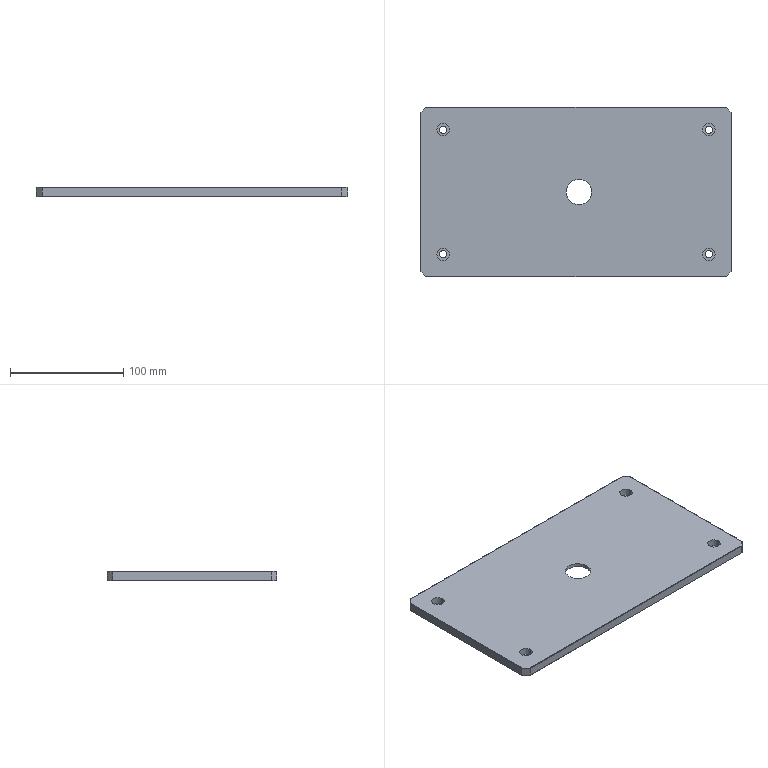Part | NX | 1 solid | 43 faces | box 275 x 150 x 8 mm | volume 300538 mm3 | plane 23 | cylinder 20 | commonest cylinder face diameters 6.4 x8 11 x8 22.5 x2 80 x2
STEP:
#1=CARTESIAN_POINT('',(0.3,4.7,0.));
#2=VERTEX_POINT('',#1);
#3=CARTESIAN_POINT('',(0.3,145.3,0.));
#4=VERTEX_POINT('',#3);
#5=CARTESIAN_POINT('',(0.3,75.,0.));
#6=DIRECTION('',(0.,1.,0.));
#7=VECTOR('',#6,1000.);
#8=LINE('',#5,#7);
#9=EDGE_CURVE('',#2,#4,#8,.T.);
#10=ORIENTED_EDGE('',*,*,#9,.T.);
#11=CARTESIAN_POINT('',(4.7,149.7,0.));
#12=VERTEX_POINT('',#11);
#13=CARTESIAN_POINT('',(5.,150.,0.));
#14=DIRECTION('',(-0.7071,-0.7071,0.));
#15=VECTOR('',#14,1000.);
#16=LINE('',#13,#15);
#17=EDGE_CURVE('',#12,#4,#16,.T.);
#18=ORIENTED_EDGE('',*,*,#17,.F.);
#19=CARTESIAN_POINT('',(270.3,149.7,0.));
#20=VERTEX_POINT('',#19);
#21=CARTESIAN_POINT('',(137.5,149.7,0.));
#22=DIRECTION('',(1.,0.,0.));
#23=VECTOR('',#22,1000.);
#24=LINE('',#21,#23);
#25=EDGE_CURVE('',#12,#20,#24,.T.);
#26=ORIENTED_EDGE('',*,*,#25,.T.);
#27=CARTESIAN_POINT('',(274.7,145.3,0.));
#28=VERTEX_POINT('',#27);
#29=CARTESIAN_POINT('',(275.,145.,0.));
#30=DIRECTION('',(-0.7071,0.7071,0.));
#31=VECTOR('',#30,1000.);
#32=LINE('',#29,#31);
#33=EDGE_CURVE('',#28,#20,#32,.T.);
#34=ORIENTED_EDGE('',*,*,#33,.F.);
#35=CARTESIAN_POINT('',(274.7,4.7,0.));
#36=VERTEX_POINT('',#35);
#37=CARTESIAN_POINT('',(274.7,75.,0.));
#38=DIRECTION('',(0.,-1.,0.));
#39=VECTOR('',#38,1000.);
#40=LINE('',#37,#39);
#41=EDGE_CURVE('',#28,#36,#40,.T.);
#42=ORIENTED_EDGE('',*,*,#41,.T.);
#43=CARTESIAN_POINT('',(270.3,0.3,0.));
#44=VERTEX_POINT('',#43);
#45=CARTESIAN_POINT('',(270.,0.,0.));
#46=DIRECTION('',(0.7071,0.7071,0.));
#47=VECTOR('',#46,1000.);
#48=LINE('',#45,#47);
#49=EDGE_CURVE('',#44,#36,#48,.T.);
#50=ORIENTED_EDGE('',*,*,#49,.F.);
#51=CARTESIAN_POINT('',(4.7,0.3,0.));
#52=VERTEX_POINT('',#51);
#53=CARTESIAN_POINT('',(137.5,0.3,0.));
#54=DIRECTION('',(-1.,0.,0.));
#55=VECTOR('',#54,1000.);
#56=LINE('',#53,#55);
#57=EDGE_CURVE('',#44,#52,#56,.T.);
#58=ORIENTED_EDGE('',*,*,#57,.T.);
#59=CARTESIAN_POINT('',(0.,5.,0.));
#60=DIRECTION('',(0.7071,-0.7071,0.));
#61=VECTOR('',#60,1000.);
#62=LINE('',#59,#61);
#63=EDGE_CURVE('',#2,#52,#62,.T.);
#64=ORIENTED_EDGE('',*,*,#63,.F.);
#65=EDGE_LOOP('',(#10,#18,#26,#34,#42,#50,#58,#64));
#66=FACE_BOUND('',#65,.T.);
#67=CARTESIAN_POINT('',(16.8,20.,0.));
#68=VERTEX_POINT('',#67);
#69=CARTESIAN_POINT('',(23.2,20.,0.));
#70=VERTEX_POINT('',#69);
#71=CARTESIAN_POINT('',(20.,20.,0.));
#72=DIRECTION('',(0.,0.,-1.));
#73=DIRECTION('',(-1.,0.,0.));
#74=AXIS2_PLACEMENT_3D('',#71,#72,#73);
#75=CIRCLE('',#74,3.2);
#76=EDGE_CURVE('',#68,#70,#75,.T.);
#77=ORIENTED_EDGE('',*,*,#76,.F.);
#78=CARTESIAN_POINT('',(20.,20.,0.));
#79=DIRECTION('',(0.,0.,-1.));
#80=DIRECTION('',(-1.,0.,0.));
#81=AXIS2_PLACEMENT_3D('',#78,#79,#80);
#82=CIRCLE('',#81,3.2);
#83=EDGE_CURVE('',#70,#68,#82,.T.);
#84=ORIENTED_EDGE('',*,*,#83,.F.);
#85=EDGE_LOOP('',(#77,#84));
#86=FACE_BOUND('',#85,.T.);
#87=CARTESIAN_POINT('',(258.2,130.,0.));
#88=VERTEX_POINT('',#87);
#89=CARTESIAN_POINT('',(251.8,130.,0.));
#90=VERTEX_POINT('',#89);
#91=CARTESIAN_POINT('',(255.,130.,0.));
#92=DIRECTION('',(0.,0.,-1.));
#93=DIRECTION('',(-1.,0.,0.));
#94=AXIS2_PLACEMENT_3D('',#91,#92,#93);
#95=CIRCLE('',#94,3.2);
#96=EDGE_CURVE('',#88,#90,#95,.T.);
#97=ORIENTED_EDGE('',*,*,#96,.F.);
#98=CARTESIAN_POINT('',(255.,130.,0.));
#99=DIRECTION('',(0.,0.,-1.));
#100=DIRECTION('',(-1.,0.,0.));
#101=AXIS2_PLACEMENT_3D('',#98,#99,#100);
#102=CIRCLE('',#101,3.2);
#103=EDGE_CURVE('',#90,#88,#102,.T.);
#104=ORIENTED_EDGE('',*,*,#103,.F.);
#105=EDGE_LOOP('',(#97,#104));
#106=FACE_BOUND('',#105,.T.);
#107=CARTESIAN_POINT('',(251.8,20.,0.));
#108=VERTEX_POINT('',#107);
#109=CARTESIAN_POINT('',(258.2,20.,0.));
#110=VERTEX_POINT('',#109);
#111=CARTESIAN_POINT('',(255.,20.,0.));
#112=DIRECTION('',(0.,0.,-1.));
#113=DIRECTION('',(-1.,0.,0.));
#114=AXIS2_PLACEMENT_3D('',#111,#112,#113);
#115=CIRCLE('',#114,3.2);
#116=EDGE_CURVE('',#108,#110,#115,.T.);
#117=ORIENTED_EDGE('',*,*,#116,.F.);
#118=CARTESIAN_POINT('',(255.,20.,0.));
#119=DIRECTION('',(0.,0.,-1.));
#120=DIRECTION('',(-1.,0.,0.));
#121=AXIS2_PLACEMENT_3D('',#118,#119,#120);
#122=CIRCLE('',#121,3.2);
#123=EDGE_CURVE('',#110,#108,#122,.T.);
#124=ORIENTED_EDGE('',*,*,#123,.F.);
#125=EDGE_LOOP('',(#117,#124));
#126=FACE_BOUND('',#125,.T.);
#127=CARTESIAN_POINT('',(180.,75.,0.));
#128=VERTEX_POINT('',#127);
#129=CARTESIAN_POINT('',(100.,75.,0.));
#130=VERTEX_POINT('',#129);
#131=CARTESIAN_POINT('',(140.,75.,0.));
#132=DIRECTION('',(0.,0.,-1.));
#133=DIRECTION('',(1.,0.,0.));
#134=AXIS2_PLACEMENT_3D('',#131,#132,#133);
#135=CIRCLE('',#134,40.);
#136=EDGE_CURVE('',#128,#130,#135,.T.);
#137=ORIENTED_EDGE('',*,*,#136,.F.);
#138=CARTESIAN_POINT('',(140.,75.,0.));
#139=DIRECTION('',(0.,0.,-1.));
#140=DIRECTION('',(1.,0.,0.));
#141=AXIS2_PLACEMENT_3D('',#138,#139,#140);
#142=CIRCLE('',#141,40.);
#143=EDGE_CURVE('',#130,#128,#142,.T.);
#144=ORIENTED_EDGE('',*,*,#143,.F.);
#145=EDGE_LOOP('',(#137,#144));
#146=FACE_BOUND('',#145,.T.);
#147=CARTESIAN_POINT('',(16.8,130.,0.));
#148=VERTEX_POINT('',#147);
#149=CARTESIAN_POINT('',(23.2,130.,0.));
#150=VERTEX_POINT('',#149);
#151=CARTESIAN_POINT('',(20.,130.,0.));
#152=DIRECTION('',(0.,0.,-1.));
#153=DIRECTION('',(-1.,0.,0.));
#154=AXIS2_PLACEMENT_3D('',#151,#152,#153);
#155=CIRCLE('',#154,3.2);
#156=EDGE_CURVE('',#148,#150,#155,.T.);
#157=ORIENTED_EDGE('',*,*,#156,.F.);
#158=CARTESIAN_POINT('',(20.,130.,0.));
#159=DIRECTION('',(0.,0.,-1.));
#160=DIRECTION('',(-1.,0.,0.));
#161=AXIS2_PLACEMENT_3D('',#158,#159,#160);
#162=CIRCLE('',#161,3.2);
#163=EDGE_CURVE('',#150,#148,#162,.T.);
#164=ORIENTED_EDGE('',*,*,#163,.F.);
#165=EDGE_LOOP('',(#157,#164));
#166=FACE_BOUND('',#165,.T.);
#167=CARTESIAN_POINT('',(0.,0.,0.));
#168=DIRECTION('',(0.,0.,1.));
#169=DIRECTION('',(1.,0.,0.));
#170=AXIS2_PLACEMENT_3D('',#167,#168,#169);
#171=PLANE('',#170);
#172=ADVANCED_FACE('',(#66,#86,#106,#126,#146,#166),#171,.F.);
#173=CARTESIAN_POINT('',(0.,5.,7.7));
#174=VERTEX_POINT('',#173);
#175=CARTESIAN_POINT('',(0.,145.,7.7));
#176=VERTEX_POINT('',#175);
#177=CARTESIAN_POINT('',(0.,75.,7.7));
#178=DIRECTION('',(0.,1.,0.));
#179=VECTOR('',#178,1000.);
#180=LINE('',#177,#179);
#181=EDGE_CURVE('',#174,#176,#180,.T.);
#182=ORIENTED_EDGE('',*,*,#181,.T.);
#183=CARTESIAN_POINT('',(0.,145.,0.3));
#184=VERTEX_POINT('',#183);
#185=CARTESIAN_POINT('',(0.,145.,8.));
#186=DIRECTION('',(0.,0.,-1.));
#187=VECTOR('',#186,1000.);
#188=LINE('',#185,#187);
#189=EDGE_CURVE('',#176,#184,#188,.T.);
#190=ORIENTED_EDGE('',*,*,#189,.T.);
#191=CARTESIAN_POINT('',(0.,5.,0.3));
#192=VERTEX_POINT('',#191);
#193=CARTESIAN_POINT('',(0.,75.,0.3));
#194=DIRECTION('',(0.,1.,0.));
#195=VECTOR('',#194,1000.);
#196=LINE('',#193,#195);
#197=EDGE_CURVE('',#192,#184,#196,.T.);
#198=ORIENTED_EDGE('',*,*,#197,.F.);
#199=CARTESIAN_POINT('',(0.,5.,8.));
#200=DIRECTION('',(0.,0.,-1.));
#201=VECTOR('',#200,1000.);
#202=LINE('',#199,#201);
#203=EDGE_CURVE('',#174,#192,#202,.T.);
#204=ORIENTED_EDGE('',*,*,#203,.F.);
#205=EDGE_LOOP('',(#182,#190,#198,#204));
#206=FACE_BOUND('',#205,.T.);
#207=CARTESIAN_POINT('',(0.,150.,0.));
#208=DIRECTION('',(-1.,0.,0.));
#209=DIRECTION('',(0.,0.,1.));
#210=AXIS2_PLACEMENT_3D('',#207,#208,#209);
#211=PLANE('',#210);
#212=ADVANCED_FACE('',(#206),#211,.T.);
#213=ORIENTED_EDGE('',*,*,#189,.F.);
#214=CARTESIAN_POINT('',(0.3,145.3,8.));
#215=VERTEX_POINT('',#214);
#216=CARTESIAN_POINT('',(-145.,0.,-137.3));
#217=DIRECTION('',(-0.5774,-0.5774,-0.5774));
#218=VECTOR('',#217,1000.);
#219=LINE('',#216,#218);
#220=EDGE_CURVE('',#215,#176,#219,.T.);
#221=ORIENTED_EDGE('',*,*,#220,.F.);
#222=CARTESIAN_POINT('',(4.7,149.7,8.));
#223=VERTEX_POINT('',#222);
#224=CARTESIAN_POINT('',(0.,145.,8.));
#225=DIRECTION('',(0.7071,0.7071,0.));
#226=VECTOR('',#225,1000.);
#227=LINE('',#224,#226);
#228=EDGE_CURVE('',#215,#223,#227,.T.);
#229=ORIENTED_EDGE('',*,*,#228,.T.);
#230=CARTESIAN_POINT('',(5.,150.,7.7));
#231=VERTEX_POINT('',#230);
#232=CARTESIAN_POINT('',(-145.,0.,157.7));
#233=DIRECTION('',(-0.5774,-0.5774,0.5774));
#234=VECTOR('',#233,1000.);
#235=LINE('',#232,#234);
#236=EDGE_CURVE('',#231,#223,#235,.T.);
#237=ORIENTED_EDGE('',*,*,#236,.F.);
#238=CARTESIAN_POINT('',(5.,150.,0.3));
#239=VERTEX_POINT('',#238);
#240=CARTESIAN_POINT('',(5.,150.,8.));
#241=DIRECTION('',(0.,0.,-1.));
#242=VECTOR('',#241,1000.);
#243=LINE('',#240,#242);
#244=EDGE_CURVE('',#231,#239,#243,.T.);
#245=ORIENTED_EDGE('',*,*,#244,.T.);
#246=CARTESIAN_POINT('',(-145.,0.,-149.7));
#247=DIRECTION('',(0.5774,0.5774,0.5774));
#248=VECTOR('',#247,1000.);
#249=LINE('',#246,#248);
#250=EDGE_CURVE('',#12,#239,#249,.T.);
#251=ORIENTED_EDGE('',*,*,#250,.F.);
#252=ORIENTED_EDGE('',*,*,#17,.T.);
#253=CARTESIAN_POINT('',(0.3,145.3,0.));
#254=DIRECTION('',(0.5774,0.5774,-0.5774));
#255=VECTOR('',#254,1000.);
#256=LINE('',#253,#255);
#257=EDGE_CURVE('',#184,#4,#256,.T.);
#258=ORIENTED_EDGE('',*,*,#257,.F.);
#259=EDGE_LOOP('',(#213,#221,#229,#237,#245,#251,#252,#258));
#260=FACE_BOUND('',#259,.T.);
#261=CARTESIAN_POINT('',(0.,145.,0.));
#262=DIRECTION('',(-0.7071,0.7071,0.));
#263=DIRECTION('',(0.,0.,1.));
#264=AXIS2_PLACEMENT_3D('',#261,#262,#263);
#265=PLANE('',#264);
#266=ADVANCED_FACE('',(#260),#265,.T.);
#267=CARTESIAN_POINT('',(270.,150.,7.7));
#268=VERTEX_POINT('',#267);
#269=CARTESIAN_POINT('',(137.5,150.,7.7));
#270=DIRECTION('',(1.,0.,0.));
#271=VECTOR('',#270,1000.);
#272=LINE('',#269,#271);
#273=EDGE_CURVE('',#231,#268,#272,.T.);
#274=ORIENTED_EDGE('',*,*,#273,.T.);
#275=CARTESIAN_POINT('',(270.,150.,0.3));
#276=VERTEX_POINT('',#275);
#277=CARTESIAN_POINT('',(270.,150.,8.));
#278=DIRECTION('',(0.,0.,-1.));
#279=VECTOR('',#278,1000.);
#280=LINE('',#277,#279);
#281=EDGE_CURVE('',#268,#276,#280,.T.);
#282=ORIENTED_EDGE('',*,*,#281,.T.);
#283=CARTESIAN_POINT('',(137.5,150.,0.3));
#284=DIRECTION('',(1.,0.,0.));
#285=VECTOR('',#284,1000.);
#286=LINE('',#283,#285);
#287=EDGE_CURVE('',#239,#276,#286,.T.);
#288=ORIENTED_EDGE('',*,*,#287,.F.);
#289=ORIENTED_EDGE('',*,*,#244,.F.);
#290=EDGE_LOOP('',(#274,#282,#288,#289));
#291=FACE_BOUND('',#290,.T.);
#292=CARTESIAN_POINT('',(275.,150.,0.));
#293=DIRECTION('',(0.,1.,0.));
#294=DIRECTION('',(1.,0.,0.));
#295=AXIS2_PLACEMENT_3D('',#292,#293,#294);
#296=PLANE('',#295);
#297=ADVANCED_FACE('',(#291),#296,.T.);
#298=ORIENTED_EDGE('',*,*,#281,.F.);
#299=CARTESIAN_POINT('',(270.3,149.7,8.));
#300=VERTEX_POINT('',#299);
#301=CARTESIAN_POINT('',(420.,0.,157.7));
#302=DIRECTION('',(-0.5774,0.5774,-0.5774));
#303=VECTOR('',#302,1000.);
#304=LINE('',#301,#303);
#305=EDGE_CURVE('',#300,#268,#304,.T.);
#306=ORIENTED_EDGE('',*,*,#305,.F.);
#307=CARTESIAN_POINT('',(274.7,145.3,8.));
#308=VERTEX_POINT('',#307);
#309=CARTESIAN_POINT('',(270.,150.,8.));
#310=DIRECTION('',(0.7071,-0.7071,0.));
#311=VECTOR('',#310,1000.);
#312=LINE('',#309,#311);
#313=EDGE_CURVE('',#300,#308,#312,.T.);
#314=ORIENTED_EDGE('',*,*,#313,.T.);
#315=CARTESIAN_POINT('',(275.,145.,7.7));
#316=VERTEX_POINT('',#315);
#317=CARTESIAN_POINT('',(420.,0.,-137.3));
#318=DIRECTION('',(-0.5774,0.5774,0.5774));
#319=VECTOR('',#318,1000.);
#320=LINE('',#317,#319);
#321=EDGE_CURVE('',#316,#308,#320,.T.);
#322=ORIENTED_EDGE('',*,*,#321,.F.);
#323=CARTESIAN_POINT('',(275.,145.,0.3));
#324=VERTEX_POINT('',#323);
#325=CARTESIAN_POINT('',(275.,145.,8.));
#326=DIRECTION('',(0.,0.,-1.));
#327=VECTOR('',#326,1000.);
#328=LINE('',#325,#327);
#329=EDGE_CURVE('',#316,#324,#328,.T.);
#330=ORIENTED_EDGE('',*,*,#329,.T.);
#331=CARTESIAN_POINT('',(420.,0.,145.3));
#332=DIRECTION('',(0.5774,-0.5774,0.5774));
#333=VECTOR('',#332,1000.);
#334=LINE('',#331,#333);
#335=EDGE_CURVE('',#28,#324,#334,.T.);
#336=ORIENTED_EDGE('',*,*,#335,.F.);
#337=ORIENTED_EDGE('',*,*,#33,.T.);
#338=CARTESIAN_POINT('',(420.,0.,-149.7));
#339=DIRECTION('',(0.5774,-0.5774,-0.5774));
#340=VECTOR('',#339,1000.);
#341=LINE('',#338,#340);
#342=EDGE_CURVE('',#276,#20,#341,.T.);
#343=ORIENTED_EDGE('',*,*,#342,.F.);
#344=EDGE_LOOP('',(#298,#306,#314,#322,#330,#336,#337,#343));
#345=FACE_BOUND('',#344,.T.);
#346=CARTESIAN_POINT('',(270.,150.,0.));
#347=DIRECTION('',(0.7071,0.7071,0.));
#348=DIRECTION('',(0.,0.,-1.));
#349=AXIS2_PLACEMENT_3D('',#346,#347,#348);
#350=PLANE('',#349);
#351=ADVANCED_FACE('',(#345),#350,.T.);
#352=CARTESIAN_POINT('',(275.,5.,7.7));
#353=VERTEX_POINT('',#352);
#354=CARTESIAN_POINT('',(275.,75.,7.7));
#355=DIRECTION('',(0.,-1.,0.));
#356=VECTOR('',#355,1000.);
#357=LINE('',#354,#356);
#358=EDGE_CURVE('',#316,#353,#357,.T.);
#359=ORIENTED_EDGE('',*,*,#358,.T.);
#360=CARTESIAN_POINT('',(275.,5.,0.3));
#361=VERTEX_POINT('',#360);
#362=CARTESIAN_POINT('',(275.,5.,8.));
#363=DIRECTION('',(0.,0.,-1.));
#364=VECTOR('',#363,1000.);
#365=LINE('',#362,#364);
#366=EDGE_CURVE('',#353,#361,#365,.T.);
#367=ORIENTED_EDGE('',*,*,#366,.T.);
#368=CARTESIAN_POINT('',(275.,75.,0.3));
#369=DIRECTION('',(0.,-1.,0.));
#370=VECTOR('',#369,1000.);
#371=LINE('',#368,#370);
#372=EDGE_CURVE('',#324,#361,#371,.T.);
#373=ORIENTED_EDGE('',*,*,#372,.F.);
#374=ORIENTED_EDGE('',*,*,#329,.F.);
#375=EDGE_LOOP('',(#359,#367,#373,#374));
#376=FACE_BOUND('',#375,.T.);
#377=CARTESIAN_POINT('',(275.,0.,0.));
#378=DIRECTION('',(1.,0.,0.));
#379=DIRECTION('',(0.,1.,0.));
#380=AXIS2_PLACEMENT_3D('',#377,#378,#379);
#381=PLANE('',#380);
#382=ADVANCED_FACE('',(#376),#381,.T.);
#383=ORIENTED_EDGE('',*,*,#366,.F.);
#384=CARTESIAN_POINT('',(274.7,4.7,8.));
#385=VERTEX_POINT('',#384);
#386=CARTESIAN_POINT('',(270.,0.,12.7));
#387=DIRECTION('',(0.5774,0.5774,-0.5774));
#388=VECTOR('',#387,1000.);
#389=LINE('',#386,#388);
#390=EDGE_CURVE('',#385,#353,#389,.T.);
#391=ORIENTED_EDGE('',*,*,#390,.F.);
#392=CARTESIAN_POINT('',(270.3,0.3,8.));
#393=VERTEX_POINT('',#392);
#394=CARTESIAN_POINT('',(275.,5.,8.));
#395=DIRECTION('',(-0.7071,-0.7071,0.));
#396=VECTOR('',#395,1000.);
#397=LINE('',#394,#396);
#398=EDGE_CURVE('',#385,#393,#397,.T.);
#399=ORIENTED_EDGE('',*,*,#398,.T.);
#400=CARTESIAN_POINT('',(270.,0.,7.7));
#401=VERTEX_POINT('',#400);
#402=CARTESIAN_POINT('',(0.,-270.,-262.3));
#403=DIRECTION('',(0.5774,0.5774,0.5774));
#404=VECTOR('',#403,1000.);
#405=LINE('',#402,#404);
#406=EDGE_CURVE('',#401,#393,#405,.T.);
#407=ORIENTED_EDGE('',*,*,#406,.F.);
#408=CARTESIAN_POINT('',(270.,0.,0.3));
#409=VERTEX_POINT('',#408);
#410=CARTESIAN_POINT('',(270.,0.,8.));
#411=DIRECTION('',(0.,0.,-1.));
#412=VECTOR('',#411,1000.);
#413=LINE('',#410,#412);
#414=EDGE_CURVE('',#401,#409,#413,.T.);
#415=ORIENTED_EDGE('',*,*,#414,.T.);
#416=CARTESIAN_POINT('',(270.3,0.3,0.));
#417=DIRECTION('',(-0.5774,-0.5774,0.5774));
#418=VECTOR('',#417,1000.);
#419=LINE('',#416,#418);
#420=EDGE_CURVE('',#44,#409,#419,.T.);
#421=ORIENTED_EDGE('',*,*,#420,.F.);
#422=ORIENTED_EDGE('',*,*,#49,.T.);
#423=CARTESIAN_POINT('',(270.,0.,-4.7));
#424=DIRECTION('',(-0.5774,-0.5774,-0.5774));
#425=VECTOR('',#424,1000.);
#426=LINE('',#423,#425);
#427=EDGE_CURVE('',#361,#36,#426,.T.);
#428=ORIENTED_EDGE('',*,*,#427,.F.);
#429=EDGE_LOOP('',(#383,#391,#399,#407,#415,#421,#422,#428));
#430=FACE_BOUND('',#429,.T.);
#431=CARTESIAN_POINT('',(275.,5.,0.));
#432=DIRECTION('',(0.7071,-0.7071,0.));
#433=DIRECTION('',(0.,0.,-1.));
#434=AXIS2_PLACEMENT_3D('',#431,#432,#433);
#435=PLANE('',#434);
#436=ADVANCED_FACE('',(#430),#435,.T.);
#437=CARTESIAN_POINT('',(5.,0.,7.7));
#438=VERTEX_POINT('',#437);
#439=CARTESIAN_POINT('',(137.5,0.,7.7));
#440=DIRECTION('',(-1.,0.,0.));
#441=VECTOR('',#440,1000.);
#442=LINE('',#439,#441);
#443=EDGE_CURVE('',#401,#438,#442,.T.);
#444=ORIENTED_EDGE('',*,*,#443,.T.);
#445=CARTESIAN_POINT('',(5.,0.,0.3));
#446=VERTEX_POINT('',#445);
#447=CARTESIAN_POINT('',(5.,0.,8.));
#448=DIRECTION('',(0.,0.,-1.));
#449=VECTOR('',#448,1000.);
#450=LINE('',#447,#449);
#451=EDGE_CURVE('',#438,#446,#450,.T.);
#452=ORIENTED_EDGE('',*,*,#451,.T.);
#453=CARTESIAN_POINT('',(137.5,0.,0.3));
#454=DIRECTION('',(-1.,0.,0.));
#455=VECTOR('',#454,1000.);
#456=LINE('',#453,#455);
#457=EDGE_CURVE('',#409,#446,#456,.T.);
#458=ORIENTED_EDGE('',*,*,#457,.F.);
#459=ORIENTED_EDGE('',*,*,#414,.F.);
#460=EDGE_LOOP('',(#444,#452,#458,#459));
#461=FACE_BOUND('',#460,.T.);
#462=CARTESIAN_POINT('',(0.,0.,0.));
#463=DIRECTION('',(0.,-1.,0.));
#464=DIRECTION('',(0.,0.,-1.));
#465=AXIS2_PLACEMENT_3D('',#462,#463,#464);
#466=PLANE('',#465);
#467=ADVANCED_FACE('',(#461),#466,.T.);
#468=ORIENTED_EDGE('',*,*,#451,.F.);
#469=CARTESIAN_POINT('',(4.7,0.3,8.));
#470=VERTEX_POINT('',#469);
#471=CARTESIAN_POINT('',(0.,5.,12.7));
#472=DIRECTION('',(0.5774,-0.5774,-0.5774));
#473=VECTOR('',#472,1000.);
#474=LINE('',#471,#473);
#475=EDGE_CURVE('',#470,#438,#474,.T.);
#476=ORIENTED_EDGE('',*,*,#475,.F.);
#477=CARTESIAN_POINT('',(0.3,4.7,8.));
#478=VERTEX_POINT('',#477);
#479=CARTESIAN_POINT('',(5.,0.,8.));
#480=DIRECTION('',(-0.7071,0.7071,0.));
#481=VECTOR('',#480,1000.);
#482=LINE('',#479,#481);
#483=EDGE_CURVE('',#470,#478,#482,.T.);
#484=ORIENTED_EDGE('',*,*,#483,.T.);
#485=CARTESIAN_POINT('',(5.,0.,12.7));
#486=DIRECTION('',(0.5774,-0.5774,0.5774));
#487=VECTOR('',#486,1000.);
#488=LINE('',#485,#487);
#489=EDGE_CURVE('',#174,#478,#488,.T.);
#490=ORIENTED_EDGE('',*,*,#489,.F.);
#491=ORIENTED_EDGE('',*,*,#203,.T.);
#492=CARTESIAN_POINT('',(0.3,4.7,0.));
#493=DIRECTION('',(-0.5774,0.5774,0.5774));
#494=VECTOR('',#493,1000.);
#495=LINE('',#492,#494);
#496=EDGE_CURVE('',#2,#192,#495,.T.);
#497=ORIENTED_EDGE('',*,*,#496,.F.);
#498=ORIENTED_EDGE('',*,*,#63,.T.);
#499=CARTESIAN_POINT('',(4.7,0.3,0.));
#500=DIRECTION('',(-0.5774,0.5774,-0.5774));
#501=VECTOR('',#500,1000.);
#502=LINE('',#499,#501);
#503=EDGE_CURVE('',#446,#52,#502,.T.);
#504=ORIENTED_EDGE('',*,*,#503,.F.);
#505=EDGE_LOOP('',(#468,#476,#484,#490,#491,#497,#498,#504));
#506=FACE_BOUND('',#505,.T.);
#507=CARTESIAN_POINT('',(5.,0.,0.));
#508=DIRECTION('',(-0.7071,-0.7071,0.));
#509=DIRECTION('',(-0.7071,0.7071,0.));
#510=AXIS2_PLACEMENT_3D('',#507,#508,#509);
#511=PLANE('',#510);
#512=ADVANCED_FACE('',(#506),#511,.T.);
#513=CARTESIAN_POINT('',(0.3,75.,8.));
#514=DIRECTION('',(0.,1.,0.));
#515=VECTOR('',#514,1000.);
#516=LINE('',#513,#515);
#517=EDGE_CURVE('',#478,#215,#516,.T.);
#518=ORIENTED_EDGE('',*,*,#517,.F.);
#519=ORIENTED_EDGE('',*,*,#483,.F.);
#520=CARTESIAN_POINT('',(137.5,0.3,8.));
#521=DIRECTION('',(-1.,0.,0.));
#522=VECTOR('',#521,1000.);
#523=LINE('',#520,#522);
#524=EDGE_CURVE('',#393,#470,#523,.T.);
#525=ORIENTED_EDGE('',*,*,#524,.F.);
#526=ORIENTED_EDGE('',*,*,#398,.F.);
#527=CARTESIAN_POINT('',(274.7,75.,8.));
#528=DIRECTION('',(0.,-1.,0.));
#529=VECTOR('',#528,1000.);
#530=LINE('',#527,#529);
#531=EDGE_CURVE('',#308,#385,#530,.T.);
#532=ORIENTED_EDGE('',*,*,#531,.F.);
#533=ORIENTED_EDGE('',*,*,#313,.F.);
#534=CARTESIAN_POINT('',(137.5,149.7,8.));
#535=DIRECTION('',(1.,0.,0.));
#536=VECTOR('',#535,1000.);
#537=LINE('',#534,#536);
#538=EDGE_CURVE('',#223,#300,#537,.T.);
#539=ORIENTED_EDGE('',*,*,#538,.F.);
#540=ORIENTED_EDGE('',*,*,#228,.F.);
#541=EDGE_LOOP('',(#518,#519,#525,#526,#532,#533,#539,#540));
#542=FACE_BOUND('',#541,.T.);
#543=CARTESIAN_POINT('',(14.5,20.,8.));
#544=VERTEX_POINT('',#543);
#545=CARTESIAN_POINT('',(25.5,20.,8.));
#546=VERTEX_POINT('',#545);
#547=CARTESIAN_POINT('',(20.,20.,8.));
#548=DIRECTION('',(0.,0.,1.));
#549=DIRECTION('',(1.,0.,0.));
#550=AXIS2_PLACEMENT_3D('',#547,#548,#549);
#551=CIRCLE('',#550,5.5);
#552=EDGE_CURVE('',#544,#546,#551,.T.);
#553=ORIENTED_EDGE('',*,*,#552,.F.);
#554=CARTESIAN_POINT('',(20.,20.,8.));
#555=DIRECTION('',(0.,0.,1.));
#556=DIRECTION('',(1.,0.,0.));
#557=AXIS2_PLACEMENT_3D('',#554,#555,#556);
#558=CIRCLE('',#557,5.5);
#559=EDGE_CURVE('',#546,#544,#558,.T.);
#560=ORIENTED_EDGE('',*,*,#559,.F.);
#561=EDGE_LOOP('',(#553,#560));
#562=FACE_BOUND('',#561,.T.);
#563=CARTESIAN_POINT('',(249.5,130.,8.));
#564=VERTEX_POINT('',#563);
#565=CARTESIAN_POINT('',(260.5,130.,8.));
#566=VERTEX_POINT('',#565);
#567=CARTESIAN_POINT('',(255.,130.,8.));
#568=DIRECTION('',(0.,0.,1.));
#569=DIRECTION('',(1.,0.,0.));
#570=AXIS2_PLACEMENT_3D('',#567,#568,#569);
#571=CIRCLE('',#570,5.5);
#572=EDGE_CURVE('',#564,#566,#571,.T.);
#573=ORIENTED_EDGE('',*,*,#572,.F.);
#574=CARTESIAN_POINT('',(255.,130.,8.));
#575=DIRECTION('',(0.,0.,1.));
#576=DIRECTION('',(1.,0.,0.));
#577=AXIS2_PLACEMENT_3D('',#574,#575,#576);
#578=CIRCLE('',#577,5.5);
#579=EDGE_CURVE('',#566,#564,#578,.T.);
#580=ORIENTED_EDGE('',*,*,#579,.F.);
#581=EDGE_LOOP('',(#573,#580));
#582=FACE_BOUND('',#581,.T.);
#583=CARTESIAN_POINT('',(249.5,20.,8.));
#584=VERTEX_POINT('',#583);
#585=CARTESIAN_POINT('',(260.5,20.,8.));
#586=VERTEX_POINT('',#585);
#587=CARTESIAN_POINT('',(255.,20.,8.));
#588=DIRECTION('',(0.,0.,1.));
#589=DIRECTION('',(1.,0.,0.));
#590=AXIS2_PLACEMENT_3D('',#587,#588,#589);
#591=CIRCLE('',#590,5.5);
#592=EDGE_CURVE('',#584,#586,#591,.T.);
#593=ORIENTED_EDGE('',*,*,#592,.F.);
#594=CARTESIAN_POINT('',(255.,20.,8.));
#595=DIRECTION('',(0.,0.,1.));
#596=DIRECTION('',(1.,0.,0.));
#597=AXIS2_PLACEMENT_3D('',#594,#595,#596);
#598=CIRCLE('',#597,5.5);
#599=EDGE_CURVE('',#586,#584,#598,.T.);
#600=ORIENTED_EDGE('',*,*,#599,.F.);
#601=EDGE_LOOP('',(#593,#600));
#602=FACE_BOUND('',#601,.T.);
#603=CARTESIAN_POINT('',(128.75,75.,8.));
#604=VERTEX_POINT('',#603);
#605=CARTESIAN_POINT('',(151.25,75.,8.));
#606=VERTEX_POINT('',#605);
#607=CARTESIAN_POINT('',(140.,75.,8.));
#608=DIRECTION('',(0.,0.,1.));
#609=DIRECTION('',(-1.,0.,0.));
#610=AXIS2_PLACEMENT_3D('',#607,#608,#609);
#611=CIRCLE('',#610,11.25);
#612=EDGE_CURVE('',#604,#606,#611,.T.);
#613=ORIENTED_EDGE('',*,*,#612,.F.);
#614=CARTESIAN_POINT('',(140.,75.,8.));
#615=DIRECTION('',(0.,0.,1.));
#616=DIRECTION('',(-1.,0.,0.));
#617=AXIS2_PLACEMENT_3D('',#614,#615,#616);
#618=CIRCLE('',#617,11.25);
#619=EDGE_CURVE('',#606,#604,#618,.T.);
#620=ORIENTED_EDGE('',*,*,#619,.F.);
#621=EDGE_LOOP('',(#613,#620));
#622=FACE_BOUND('',#621,.T.);
#623=CARTESIAN_POINT('',(25.5,130.,8.));
#624=VERTEX_POINT('',#623);
#625=CARTESIAN_POINT('',(14.5,130.,8.));
#626=VERTEX_POINT('',#625);
#627=CARTESIAN_POINT('',(20.,130.,8.));
#628=DIRECTION('',(0.,0.,1.));
#629=DIRECTION('',(1.,0.,0.));
#630=AXIS2_PLACEMENT_3D('',#627,#628,#629);
#631=CIRCLE('',#630,5.5);
#632=EDGE_CURVE('',#624,#626,#631,.T.);
#633=ORIENTED_EDGE('',*,*,#632,.F.);
#634=CARTESIAN_POINT('',(20.,130.,8.));
#635=DIRECTION('',(0.,0.,1.));
#636=DIRECTION('',(1.,0.,0.));
#637=AXIS2_PLACEMENT_3D('',#634,#635,#636);
#638=CIRCLE('',#637,5.5);
#639=EDGE_CURVE('',#626,#624,#638,.T.);
#640=ORIENTED_EDGE('',*,*,#639,.F.);
#641=EDGE_LOOP('',(#633,#640));
#642=FACE_BOUND('',#641,.T.);
#643=CARTESIAN_POINT('',(0.,0.,8.));
#644=DIRECTION('',(0.,0.,1.));
#645=DIRECTION('',(1.,0.,0.));
#646=AXIS2_PLACEMENT_3D('',#643,#644,#645);
#647=PLANE('',#646);
#648=ADVANCED_FACE('',(#542,#562,#582,#602,#622,#642),#647,.T.);
#649=ORIENTED_EDGE('',*,*,#632,.T.);
#650=CARTESIAN_POINT('',(14.5,130.,1.5));
#651=VERTEX_POINT('',#650);
#652=CARTESIAN_POINT('',(14.5,130.,-1.24));
#653=DIRECTION('',(0.,0.,1.));
#654=VECTOR('',#653,1000.);
#655=LINE('',#652,#654);
#656=EDGE_CURVE('',#626,#651,#655,.F.);
#657=ORIENTED_EDGE('',*,*,#656,.T.);
#658=CARTESIAN_POINT('',(25.5,130.,1.5));
#659=VERTEX_POINT('',#658);
#660=CARTESIAN_POINT('',(20.,130.,1.5));
#661=DIRECTION('',(0.,0.,-1.));
#662=DIRECTION('',(1.,0.,0.));
#663=AXIS2_PLACEMENT_3D('',#660,#661,#662);
#664=CIRCLE('',#663,5.5);
#665=EDGE_CURVE('',#651,#659,#664,.T.);
#666=ORIENTED_EDGE('',*,*,#665,.T.);
#667=CARTESIAN_POINT('',(25.5,130.,-1.24));
#668=DIRECTION('',(0.,0.,1.));
#669=VECTOR('',#668,1000.);
#670=LINE('',#667,#669);
#671=EDGE_CURVE('',#624,#659,#670,.F.);
#672=ORIENTED_EDGE('',*,*,#671,.F.);
#673=EDGE_LOOP('',(#649,#657,#666,#672));
#674=FACE_BOUND('',#673,.T.);
#675=CARTESIAN_POINT('',(20.,130.,-1.24));
#676=DIRECTION('',(0.,0.,1.));
#677=DIRECTION('',(-1.,0.,0.));
#678=AXIS2_PLACEMENT_3D('',#675,#676,#677);
#679=CYLINDRICAL_SURFACE('',#678,5.5);
#680=ADVANCED_FACE('',(#674),#679,.F.);
#681=ORIENTED_EDGE('',*,*,#136,.T.);
#682=CARTESIAN_POINT('',(100.,75.,5.));
#683=VERTEX_POINT('',#682);
#684=CARTESIAN_POINT('',(100.,75.,0.));
#685=DIRECTION('',(0.,0.,1.));
#686=VECTOR('',#685,1000.);
#687=LINE('',#684,#686);
#688=EDGE_CURVE('',#683,#130,#687,.F.);
#689=ORIENTED_EDGE('',*,*,#688,.F.);
#690=CARTESIAN_POINT('',(180.,75.,5.));
#691=VERTEX_POINT('',#690);
#692=CARTESIAN_POINT('',(140.,75.,5.));
#693=DIRECTION('',(0.,0.,1.));
#694=DIRECTION('',(-1.,0.,0.));
#695=AXIS2_PLACEMENT_3D('',#692,#693,#694);
#696=CIRCLE('',#695,40.);
#697=EDGE_CURVE('',#683,#691,#696,.T.);
#698=ORIENTED_EDGE('',*,*,#697,.T.);
#699=CARTESIAN_POINT('',(180.,75.,0.));
#700=DIRECTION('',(0.,0.,1.));
#701=VECTOR('',#700,1000.);
#702=LINE('',#699,#701);
#703=EDGE_CURVE('',#691,#128,#702,.F.);
#704=ORIENTED_EDGE('',*,*,#703,.T.);
#705=EDGE_LOOP('',(#681,#689,#698,#704));
#706=FACE_BOUND('',#705,.T.);
#707=CARTESIAN_POINT('',(140.,75.,0.));
#708=DIRECTION('',(0.,0.,1.));
#709=DIRECTION('',(1.,0.,0.));
#710=AXIS2_PLACEMENT_3D('',#707,#708,#709);
#711=CYLINDRICAL_SURFACE('',#710,40.);
#712=ADVANCED_FACE('',(#706),#711,.F.);
#713=ORIENTED_EDGE('',*,*,#665,.F.);
#714=CARTESIAN_POINT('',(20.,130.,1.5));
#715=DIRECTION('',(0.,0.,-1.));
#716=DIRECTION('',(1.,0.,0.));
#717=AXIS2_PLACEMENT_3D('',#714,#715,#716);
#718=CIRCLE('',#717,5.5);
#719=EDGE_CURVE('',#659,#651,#718,.T.);
#720=ORIENTED_EDGE('',*,*,#719,.F.);
#721=EDGE_LOOP('',(#713,#720));
#722=FACE_BOUND('',#721,.T.);
#723=CARTESIAN_POINT('',(16.8,130.,1.5));
#724=VERTEX_POINT('',#723);
#725=CARTESIAN_POINT('',(23.2,130.,1.5));
#726=VERTEX_POINT('',#725);
#727=CARTESIAN_POINT('',(20.,130.,1.5));
#728=DIRECTION('',(0.,0.,1.));
#729=DIRECTION('',(-1.,0.,0.));
#730=AXIS2_PLACEMENT_3D('',#727,#728,#729);
#731=CIRCLE('',#730,3.2);
#732=EDGE_CURVE('',#724,#726,#731,.T.);
#733=ORIENTED_EDGE('',*,*,#732,.F.);
#734=CARTESIAN_POINT('',(20.,130.,1.5));
#735=DIRECTION('',(0.,0.,1.));
#736=DIRECTION('',(-1.,0.,0.));
#737=AXIS2_PLACEMENT_3D('',#734,#735,#736);
#738=CIRCLE('',#737,3.2);
#739=EDGE_CURVE('',#726,#724,#738,.T.);
#740=ORIENTED_EDGE('',*,*,#739,.F.);
#741=EDGE_LOOP('',(#733,#740));
#742=FACE_BOUND('',#741,.T.);
#743=CARTESIAN_POINT('',(20.,130.,1.5));
#744=DIRECTION('',(0.,0.,1.));
#745=DIRECTION('',(1.,0.,0.));
#746=AXIS2_PLACEMENT_3D('',#743,#744,#745);
#747=PLANE('',#746);
#748=ADVANCED_FACE('',(#722,#742),#747,.T.);
#749=ORIENTED_EDGE('',*,*,#732,.T.);
#750=CARTESIAN_POINT('',(23.2,130.,-1.24));
#751=DIRECTION('',(0.,0.,1.));
#752=VECTOR('',#751,1000.);
#753=LINE('',#750,#752);
#754=EDGE_CURVE('',#150,#726,#753,.T.);
#755=ORIENTED_EDGE('',*,*,#754,.F.);
#756=ORIENTED_EDGE('',*,*,#163,.T.);
#757=CARTESIAN_POINT('',(16.8,130.,-1.24));
#758=DIRECTION('',(0.,0.,1.));
#759=VECTOR('',#758,1000.);
#760=LINE('',#757,#759);
#761=EDGE_CURVE('',#148,#724,#760,.T.);
#762=ORIENTED_EDGE('',*,*,#761,.T.);
#763=EDGE_LOOP('',(#749,#755,#756,#762));
#764=FACE_BOUND('',#763,.T.);
#765=CARTESIAN_POINT('',(20.,130.,-1.24));
#766=DIRECTION('',(0.,0.,1.));
#767=DIRECTION('',(-1.,0.,0.));
#768=AXIS2_PLACEMENT_3D('',#765,#766,#767);
#769=CYLINDRICAL_SURFACE('',#768,3.2);
#770=ADVANCED_FACE('',(#764),#769,.F.);
#771=CARTESIAN_POINT('',(260.5,20.,1.5));
#772=VERTEX_POINT('',#771);
#773=CARTESIAN_POINT('',(249.5,20.,1.5));
#774=VERTEX_POINT('',#773);
#775=CARTESIAN_POINT('',(255.,20.,1.5));
#776=DIRECTION('',(0.,0.,-1.));
#777=DIRECTION('',(-1.,0.,0.));
#778=AXIS2_PLACEMENT_3D('',#775,#776,#777);
#779=CIRCLE('',#778,5.5);
#780=EDGE_CURVE('',#772,#774,#779,.T.);
#781=ORIENTED_EDGE('',*,*,#780,.F.);
#782=CARTESIAN_POINT('',(255.,20.,1.5));
#783=DIRECTION('',(0.,0.,-1.));
#784=DIRECTION('',(-1.,0.,0.));
#785=AXIS2_PLACEMENT_3D('',#782,#783,#784);
#786=CIRCLE('',#785,5.5);
#787=EDGE_CURVE('',#774,#772,#786,.T.);
#788=ORIENTED_EDGE('',*,*,#787,.F.);
#789=EDGE_LOOP('',(#781,#788));
#790=FACE_BOUND('',#789,.T.);
#791=CARTESIAN_POINT('',(258.2,20.,1.5));
#792=VERTEX_POINT('',#791);
#793=CARTESIAN_POINT('',(251.8,20.,1.5));
#794=VERTEX_POINT('',#793);
#795=CARTESIAN_POINT('',(255.,20.,1.5));
#796=DIRECTION('',(0.,0.,1.));
#797=DIRECTION('',(-1.,0.,0.));
#798=AXIS2_PLACEMENT_3D('',#795,#796,#797);
#799=CIRCLE('',#798,3.2);
#800=EDGE_CURVE('',#792,#794,#799,.T.);
#801=ORIENTED_EDGE('',*,*,#800,.F.);
#802=CARTESIAN_POINT('',(255.,20.,1.5));
#803=DIRECTION('',(0.,0.,1.));
#804=DIRECTION('',(-1.,0.,0.));
#805=AXIS2_PLACEMENT_3D('',#802,#803,#804);
#806=CIRCLE('',#805,3.2);
#807=EDGE_CURVE('',#794,#792,#806,.T.);
#808=ORIENTED_EDGE('',*,*,#807,.F.);
#809=EDGE_LOOP('',(#801,#808));
#810=FACE_BOUND('',#809,.T.);
#811=CARTESIAN_POINT('',(255.,20.,1.5));
#812=DIRECTION('',(0.,0.,1.));
#813=DIRECTION('',(1.,0.,0.));
#814=AXIS2_PLACEMENT_3D('',#811,#812,#813);
#815=PLANE('',#814);
#816=ADVANCED_FACE('',(#790,#810),#815,.T.);
#817=CARTESIAN_POINT('',(14.5,20.,1.5));
#818=VERTEX_POINT('',#817);
#819=CARTESIAN_POINT('',(25.5,20.,1.5));
#820=VERTEX_POINT('',#819);
#821=CARTESIAN_POINT('',(20.,20.,1.5));
#822=DIRECTION('',(0.,0.,-1.));
#823=DIRECTION('',(1.,0.,0.));
#824=AXIS2_PLACEMENT_3D('',#821,#822,#823);
#825=CIRCLE('',#824,5.5);
#826=EDGE_CURVE('',#818,#820,#825,.T.);
#827=ORIENTED_EDGE('',*,*,#826,.T.);
#828=CARTESIAN_POINT('',(25.5,20.,-1.24));
#829=DIRECTION('',(0.,0.,1.));
#830=VECTOR('',#829,1000.);
#831=LINE('',#828,#830);
#832=EDGE_CURVE('',#820,#546,#831,.T.);
#833=ORIENTED_EDGE('',*,*,#832,.T.);
#834=ORIENTED_EDGE('',*,*,#559,.T.);
#835=CARTESIAN_POINT('',(14.5,20.,-1.24));
#836=DIRECTION('',(0.,0.,1.));
#837=VECTOR('',#836,1000.);
#838=LINE('',#835,#837);
#839=EDGE_CURVE('',#818,#544,#838,.T.);
#840=ORIENTED_EDGE('',*,*,#839,.F.);
#841=EDGE_LOOP('',(#827,#833,#834,#840));
#842=FACE_BOUND('',#841,.T.);
#843=CARTESIAN_POINT('',(20.,20.,-1.24));
#844=DIRECTION('',(0.,0.,1.));
#845=DIRECTION('',(-1.,0.,0.));
#846=AXIS2_PLACEMENT_3D('',#843,#844,#845);
#847=CYLINDRICAL_SURFACE('',#846,5.5);
#848=ADVANCED_FACE('',(#842),#847,.F.);
#849=ORIENTED_EDGE('',*,*,#592,.T.);
#850=CARTESIAN_POINT('',(260.5,20.,-1.24));
#851=DIRECTION('',(0.,0.,1.));
#852=VECTOR('',#851,1000.);
#853=LINE('',#850,#852);
#854=EDGE_CURVE('',#586,#772,#853,.F.);
#855=ORIENTED_EDGE('',*,*,#854,.T.);
#856=ORIENTED_EDGE('',*,*,#780,.T.);
#857=CARTESIAN_POINT('',(249.5,20.,-1.24));
#858=DIRECTION('',(0.,0.,1.));
#859=VECTOR('',#858,1000.);
#860=LINE('',#857,#859);
#861=EDGE_CURVE('',#584,#774,#860,.F.);
#862=ORIENTED_EDGE('',*,*,#861,.F.);
#863=EDGE_LOOP('',(#849,#855,#856,#862));
#864=FACE_BOUND('',#863,.T.);
#865=CARTESIAN_POINT('',(255.,20.,-1.24));
#866=DIRECTION('',(0.,0.,1.));
#867=DIRECTION('',(-1.,0.,0.));
#868=AXIS2_PLACEMENT_3D('',#865,#866,#867);
#869=CYLINDRICAL_SURFACE('',#868,5.5);
#870=ADVANCED_FACE('',(#864),#869,.F.);
#871=ORIENTED_EDGE('',*,*,#826,.F.);
#872=CARTESIAN_POINT('',(20.,20.,1.5));
#873=DIRECTION('',(0.,0.,-1.));
#874=DIRECTION('',(1.,0.,0.));
#875=AXIS2_PLACEMENT_3D('',#872,#873,#874);
#876=CIRCLE('',#875,5.5);
#877=EDGE_CURVE('',#820,#818,#876,.T.);
#878=ORIENTED_EDGE('',*,*,#877,.F.);
#879=EDGE_LOOP('',(#871,#878));
#880=FACE_BOUND('',#879,.T.);
#881=CARTESIAN_POINT('',(23.2,20.,1.5));
#882=VERTEX_POINT('',#881);
#883=CARTESIAN_POINT('',(16.8,20.,1.5));
#884=VERTEX_POINT('',#883);
#885=CARTESIAN_POINT('',(20.,20.,1.5));
#886=DIRECTION('',(0.,0.,1.));
#887=DIRECTION('',(-1.,0.,0.));
#888=AXIS2_PLACEMENT_3D('',#885,#886,#887);
#889=CIRCLE('',#888,3.2);
#890=EDGE_CURVE('',#882,#884,#889,.T.);
#891=ORIENTED_EDGE('',*,*,#890,.F.);
#892=CARTESIAN_POINT('',(20.,20.,1.5));
#893=DIRECTION('',(0.,0.,1.));
#894=DIRECTION('',(-1.,0.,0.));
#895=AXIS2_PLACEMENT_3D('',#892,#893,#894);
#896=CIRCLE('',#895,3.2);
#897=EDGE_CURVE('',#884,#882,#896,.T.);
#898=ORIENTED_EDGE('',*,*,#897,.F.);
#899=EDGE_LOOP('',(#891,#898));
#900=FACE_BOUND('',#899,.T.);
#901=CARTESIAN_POINT('',(20.,20.,1.5));
#902=DIRECTION('',(0.,0.,1.));
#903=DIRECTION('',(1.,0.,0.));
#904=AXIS2_PLACEMENT_3D('',#901,#902,#903);
#905=PLANE('',#904);
#906=ADVANCED_FACE('',(#880,#900),#905,.T.);
#907=ORIENTED_EDGE('',*,*,#890,.T.);
#908=CARTESIAN_POINT('',(16.8,20.,-1.24));
#909=DIRECTION('',(0.,0.,1.));
#910=VECTOR('',#909,1000.);
#911=LINE('',#908,#910);
#912=EDGE_CURVE('',#884,#68,#911,.F.);
#913=ORIENTED_EDGE('',*,*,#912,.T.);
#914=ORIENTED_EDGE('',*,*,#76,.T.);
#915=CARTESIAN_POINT('',(23.2,20.,-1.24));
#916=DIRECTION('',(0.,0.,1.));
#917=VECTOR('',#916,1000.);
#918=LINE('',#915,#917);
#919=EDGE_CURVE('',#882,#70,#918,.F.);
#920=ORIENTED_EDGE('',*,*,#919,.F.);
#921=EDGE_LOOP('',(#907,#913,#914,#920));
#922=FACE_BOUND('',#921,.T.);
#923=CARTESIAN_POINT('',(20.,20.,-1.24));
#924=DIRECTION('',(0.,0.,1.));
#925=DIRECTION('',(-1.,0.,0.));
#926=AXIS2_PLACEMENT_3D('',#923,#924,#925);
#927=CYLINDRICAL_SURFACE('',#926,3.2);
#928=ADVANCED_FACE('',(#922),#927,.F.);
#929=ORIENTED_EDGE('',*,*,#612,.T.);
#930=CARTESIAN_POINT('',(151.25,75.,5.));
#931=VERTEX_POINT('',#930);
#932=CARTESIAN_POINT('',(151.25,75.,8.));
#933=DIRECTION('',(0.,0.,1.));
#934=VECTOR('',#933,1000.);
#935=LINE('',#932,#934);
#936=EDGE_CURVE('',#931,#606,#935,.T.);
#937=ORIENTED_EDGE('',*,*,#936,.F.);
#938=CARTESIAN_POINT('',(128.75,75.,5.));
#939=VERTEX_POINT('',#938);
#940=CARTESIAN_POINT('',(140.,75.,5.));
#941=DIRECTION('',(0.,0.,-1.));
#942=DIRECTION('',(1.,0.,0.));
#943=AXIS2_PLACEMENT_3D('',#940,#941,#942);
#944=CIRCLE('',#943,11.25);
#945=EDGE_CURVE('',#931,#939,#944,.T.);
#946=ORIENTED_EDGE('',*,*,#945,.T.);
#947=CARTESIAN_POINT('',(128.75,75.,8.));
#948=DIRECTION('',(0.,0.,1.));
#949=VECTOR('',#948,1000.);
#950=LINE('',#947,#949);
#951=EDGE_CURVE('',#939,#604,#950,.T.);
#952=ORIENTED_EDGE('',*,*,#951,.T.);
#953=EDGE_LOOP('',(#929,#937,#946,#952));
#954=FACE_BOUND('',#953,.T.);
#955=CARTESIAN_POINT('',(140.,75.,8.));
#956=DIRECTION('',(0.,0.,1.));
#957=DIRECTION('',(1.,0.,0.));
#958=AXIS2_PLACEMENT_3D('',#955,#956,#957);
#959=CYLINDRICAL_SURFACE('',#958,11.25);
#960=ADVANCED_FACE('',(#954),#959,.F.);
#961=ORIENTED_EDGE('',*,*,#572,.T.);
#962=CARTESIAN_POINT('',(260.5,130.,1.5));
#963=VERTEX_POINT('',#962);
#964=CARTESIAN_POINT('',(260.5,130.,-1.24));
#965=DIRECTION('',(0.,0.,1.));
#966=VECTOR('',#965,1000.);
#967=LINE('',#964,#966);
#968=EDGE_CURVE('',#963,#566,#967,.T.);
#969=ORIENTED_EDGE('',*,*,#968,.F.);
#970=CARTESIAN_POINT('',(249.5,130.,1.5));
#971=VERTEX_POINT('',#970);
#972=CARTESIAN_POINT('',(255.,130.,1.5));
#973=DIRECTION('',(0.,0.,-1.));
#974=DIRECTION('',(1.,0.,0.));
#975=AXIS2_PLACEMENT_3D('',#972,#973,#974);
#976=CIRCLE('',#975,5.5);
#977=EDGE_CURVE('',#963,#971,#976,.T.);
#978=ORIENTED_EDGE('',*,*,#977,.T.);
#979=CARTESIAN_POINT('',(249.5,130.,-1.24));
#980=DIRECTION('',(0.,0.,1.));
#981=VECTOR('',#980,1000.);
#982=LINE('',#979,#981);
#983=EDGE_CURVE('',#971,#564,#982,.T.);
#984=ORIENTED_EDGE('',*,*,#983,.T.);
#985=EDGE_LOOP('',(#961,#969,#978,#984));
#986=FACE_BOUND('',#985,.T.);
#987=CARTESIAN_POINT('',(255.,130.,-1.24));
#988=DIRECTION('',(0.,0.,1.));
#989=DIRECTION('',(-1.,0.,0.));
#990=AXIS2_PLACEMENT_3D('',#987,#988,#989);
#991=CYLINDRICAL_SURFACE('',#990,5.5);
#992=ADVANCED_FACE('',(#986),#991,.F.);
#993=ORIENTED_EDGE('',*,*,#800,.T.);
#994=CARTESIAN_POINT('',(251.8,20.,-1.24));
#995=DIRECTION('',(0.,0.,1.));
#996=VECTOR('',#995,1000.);
#997=LINE('',#994,#996);
#998=EDGE_CURVE('',#794,#108,#997,.F.);
#999=ORIENTED_EDGE('',*,*,#998,.T.);
#1000=ORIENTED_EDGE('',*,*,#116,.T.);
#1001=CARTESIAN_POINT('',(258.2,20.,-1.24));
#1002=DIRECTION('',(0.,0.,1.));
#1003=VECTOR('',#1002,1000.);
#1004=LINE('',#1001,#1003);
#1005=EDGE_CURVE('',#792,#110,#1004,.F.);
#1006=ORIENTED_EDGE('',*,*,#1005,.F.);
#1007=EDGE_LOOP('',(#993,#999,#1000,#1006));
#1008=FACE_BOUND('',#1007,.T.);
#1009=CARTESIAN_POINT('',(255.,20.,-1.24));
#1010=DIRECTION('',(0.,0.,1.));
#1011=DIRECTION('',(-1.,0.,0.));
#1012=AXIS2_PLACEMENT_3D('',#1009,#1010,#1011);
#1013=CYLINDRICAL_SURFACE('',#1012,3.2);
#1014=ADVANCED_FACE('',(#1008),#1013,.F.);
#1015=CARTESIAN_POINT('',(255.,130.,1.5));
#1016=DIRECTION('',(0.,0.,-1.));
#1017=DIRECTION('',(1.,0.,0.));
#1018=AXIS2_PLACEMENT_3D('',#1015,#1016,#1017);
#1019=CIRCLE('',#1018,5.5);
#1020=EDGE_CURVE('',#971,#963,#1019,.T.);
#1021=ORIENTED_EDGE('',*,*,#1020,.F.);
#1022=ORIENTED_EDGE('',*,*,#977,.F.);
#1023=EDGE_LOOP('',(#1021,#1022));
#1024=FACE_BOUND('',#1023,.T.);
#1025=CARTESIAN_POINT('',(258.2,130.,1.5));
#1026=VERTEX_POINT('',#1025);
#1027=CARTESIAN_POINT('',(251.8,130.,1.5));
#1028=VERTEX_POINT('',#1027);
#1029=CARTESIAN_POINT('',(255.,130.,1.5));
#1030=DIRECTION('',(0.,0.,1.));
#1031=DIRECTION('',(-1.,0.,0.));
#1032=AXIS2_PLACEMENT_3D('',#1029,#1030,#1031);
#1033=CIRCLE('',#1032,3.2);
#1034=EDGE_CURVE('',#1026,#1028,#1033,.T.);
#1035=ORIENTED_EDGE('',*,*,#1034,.F.);
#1036=CARTESIAN_POINT('',(255.,130.,1.5));
#1037=DIRECTION('',(0.,0.,1.));
#1038=DIRECTION('',(-1.,0.,0.));
#1039=AXIS2_PLACEMENT_3D('',#1036,#1037,#1038);
#1040=CIRCLE('',#1039,3.2);
#1041=EDGE_CURVE('',#1028,#1026,#1040,.T.);
#1042=ORIENTED_EDGE('',*,*,#1041,.F.);
#1043=EDGE_LOOP('',(#1035,#1042));
#1044=FACE_BOUND('',#1043,.T.);
#1045=CARTESIAN_POINT('',(255.,130.,1.5));
#1046=DIRECTION('',(0.,0.,1.));
#1047=DIRECTION('',(1.,0.,0.));
#1048=AXIS2_PLACEMENT_3D('',#1045,#1046,#1047);
#1049=PLANE('',#1048);
#1050=ADVANCED_FACE('',(#1024,#1044),#1049,.T.);
#1051=ORIENTED_EDGE('',*,*,#96,.T.);
#1052=CARTESIAN_POINT('',(251.8,130.,-1.24));
#1053=DIRECTION('',(0.,0.,1.));
#1054=VECTOR('',#1053,1000.);
#1055=LINE('',#1052,#1054);
#1056=EDGE_CURVE('',#1028,#90,#1055,.F.);
#1057=ORIENTED_EDGE('',*,*,#1056,.F.);
#1058=ORIENTED_EDGE('',*,*,#1041,.T.);
#1059=CARTESIAN_POINT('',(258.2,130.,-1.24));
#1060=DIRECTION('',(0.,0.,1.));
#1061=VECTOR('',#1060,1000.);
#1062=LINE('',#1059,#1061);
#1063=EDGE_CURVE('',#1026,#88,#1062,.F.);
#1064=ORIENTED_EDGE('',*,*,#1063,.T.);
#1065=EDGE_LOOP('',(#1051,#1057,#1058,#1064));
#1066=FACE_BOUND('',#1065,.T.);
#1067=CARTESIAN_POINT('',(255.,130.,-1.24));
#1068=DIRECTION('',(0.,0.,1.));
#1069=DIRECTION('',(-1.,0.,0.));
#1070=AXIS2_PLACEMENT_3D('',#1067,#1068,#1069);
#1071=CYLINDRICAL_SURFACE('',#1070,3.2);
#1072=ADVANCED_FACE('',(#1066),#1071,.F.);
#1073=CARTESIAN_POINT('',(140.,75.,5.));
#1074=DIRECTION('',(0.,0.,1.));
#1075=DIRECTION('',(-1.,0.,0.));
#1076=AXIS2_PLACEMENT_3D('',#1073,#1074,#1075);
#1077=CIRCLE('',#1076,40.);
#1078=EDGE_CURVE('',#691,#683,#1077,.T.);
#1079=ORIENTED_EDGE('',*,*,#1078,.F.);
#1080=ORIENTED_EDGE('',*,*,#697,.F.);
#1081=EDGE_LOOP('',(#1079,#1080));
#1082=FACE_BOUND('',#1081,.T.);
#1083=ORIENTED_EDGE('',*,*,#945,.F.);
#1084=CARTESIAN_POINT('',(140.,75.,5.));
#1085=DIRECTION('',(0.,0.,-1.));
#1086=DIRECTION('',(1.,0.,0.));
#1087=AXIS2_PLACEMENT_3D('',#1084,#1085,#1086);
#1088=CIRCLE('',#1087,11.25);
#1089=EDGE_CURVE('',#939,#931,#1088,.T.);
#1090=ORIENTED_EDGE('',*,*,#1089,.F.);
#1091=EDGE_LOOP('',(#1083,#1090));
#1092=FACE_BOUND('',#1091,.T.);
#1093=CARTESIAN_POINT('',(140.,75.,5.));
#1094=DIRECTION('',(0.,0.,1.));
#1095=DIRECTION('',(1.,0.,0.));
#1096=AXIS2_PLACEMENT_3D('',#1093,#1094,#1095);
#1097=PLANE('',#1096);
#1098=ADVANCED_FACE('',(#1082,#1092),#1097,.F.);
#1099=ORIENTED_EDGE('',*,*,#25,.F.);
#1100=ORIENTED_EDGE('',*,*,#250,.T.);
#1101=ORIENTED_EDGE('',*,*,#287,.T.);
#1102=ORIENTED_EDGE('',*,*,#342,.T.);
#1103=EDGE_LOOP('',(#1099,#1100,#1101,#1102));
#1104=FACE_BOUND('',#1103,.T.);
#1105=CARTESIAN_POINT('',(137.5,149.85,0.15));
#1106=DIRECTION('',(0.,0.7071,-0.7071));
#1107=DIRECTION('',(-1.,0.,0.));
#1108=AXIS2_PLACEMENT_3D('',#1105,#1106,#1107);
#1109=PLANE('',#1108);
#1110=ADVANCED_FACE('',(#1104),#1109,.T.);
#1111=ORIENTED_EDGE('',*,*,#273,.F.);
#1112=ORIENTED_EDGE('',*,*,#236,.T.);
#1113=ORIENTED_EDGE('',*,*,#538,.T.);
#1114=ORIENTED_EDGE('',*,*,#305,.T.);
#1115=EDGE_LOOP('',(#1111,#1112,#1113,#1114));
#1116=FACE_BOUND('',#1115,.T.);
#1117=CARTESIAN_POINT('',(137.5,149.85,7.85));
#1118=DIRECTION('',(0.,0.7071,0.7071));
#1119=DIRECTION('',(1.,0.,0.));
#1120=AXIS2_PLACEMENT_3D('',#1117,#1118,#1119);
#1121=PLANE('',#1120);
#1122=ADVANCED_FACE('',(#1116),#1121,.T.);
#1123=ORIENTED_EDGE('',*,*,#358,.F.);
#1124=ORIENTED_EDGE('',*,*,#321,.T.);
#1125=ORIENTED_EDGE('',*,*,#531,.T.);
#1126=ORIENTED_EDGE('',*,*,#390,.T.);
#1127=EDGE_LOOP('',(#1123,#1124,#1125,#1126));
#1128=FACE_BOUND('',#1127,.T.);
#1129=CARTESIAN_POINT('',(274.85,75.,7.85));
#1130=DIRECTION('',(0.7071,0.,0.7071));
#1131=DIRECTION('',(0.,-1.,0.));
#1132=AXIS2_PLACEMENT_3D('',#1129,#1130,#1131);
#1133=PLANE('',#1132);
#1134=ADVANCED_FACE('',(#1128),#1133,.T.);
#1135=ORIENTED_EDGE('',*,*,#41,.F.);
#1136=ORIENTED_EDGE('',*,*,#335,.T.);
#1137=ORIENTED_EDGE('',*,*,#372,.T.);
#1138=ORIENTED_EDGE('',*,*,#427,.T.);
#1139=EDGE_LOOP('',(#1135,#1136,#1137,#1138));
#1140=FACE_BOUND('',#1139,.T.);
#1141=CARTESIAN_POINT('',(274.85,75.,0.15));
#1142=DIRECTION('',(0.7071,0.,-0.7071));
#1143=DIRECTION('',(0.,-1.,0.));
#1144=AXIS2_PLACEMENT_3D('',#1141,#1142,#1143);
#1145=PLANE('',#1144);
#1146=ADVANCED_FACE('',(#1140),#1145,.T.);
#1147=ORIENTED_EDGE('',*,*,#57,.F.);
#1148=ORIENTED_EDGE('',*,*,#420,.T.);
#1149=ORIENTED_EDGE('',*,*,#457,.T.);
#1150=ORIENTED_EDGE('',*,*,#503,.T.);
#1151=EDGE_LOOP('',(#1147,#1148,#1149,#1150));
#1152=FACE_BOUND('',#1151,.T.);
#1153=CARTESIAN_POINT('',(137.5,0.15,0.15));
#1154=DIRECTION('',(0.,-0.7071,-0.7071));
#1155=DIRECTION('',(0.,-0.7071,0.7071));
#1156=AXIS2_PLACEMENT_3D('',#1153,#1154,#1155);
#1157=PLANE('',#1156);
#1158=ADVANCED_FACE('',(#1152),#1157,.T.);
#1159=ORIENTED_EDGE('',*,*,#443,.F.);
#1160=ORIENTED_EDGE('',*,*,#406,.T.);
#1161=ORIENTED_EDGE('',*,*,#524,.T.);
#1162=ORIENTED_EDGE('',*,*,#475,.T.);
#1163=EDGE_LOOP('',(#1159,#1160,#1161,#1162));
#1164=FACE_BOUND('',#1163,.T.);
#1165=CARTESIAN_POINT('',(137.5,0.15,7.85));
#1166=DIRECTION('',(0.,-0.7071,0.7071));
#1167=DIRECTION('',(-1.,0.,0.));
#1168=AXIS2_PLACEMENT_3D('',#1165,#1166,#1167);
#1169=PLANE('',#1168);
#1170=ADVANCED_FACE('',(#1164),#1169,.T.);
#1171=ORIENTED_EDGE('',*,*,#181,.F.);
#1172=ORIENTED_EDGE('',*,*,#489,.T.);
#1173=ORIENTED_EDGE('',*,*,#517,.T.);
#1174=ORIENTED_EDGE('',*,*,#220,.T.);
#1175=EDGE_LOOP('',(#1171,#1172,#1173,#1174));
#1176=FACE_BOUND('',#1175,.T.);
#1177=CARTESIAN_POINT('',(0.15,75.,7.85));
#1178=DIRECTION('',(-0.7071,0.,0.7071));
#1179=DIRECTION('',(0.,1.,0.));
#1180=AXIS2_PLACEMENT_3D('',#1177,#1178,#1179);
#1181=PLANE('',#1180);
#1182=ADVANCED_FACE('',(#1176),#1181,.T.);
#1183=ORIENTED_EDGE('',*,*,#9,.F.);
#1184=ORIENTED_EDGE('',*,*,#496,.T.);
#1185=ORIENTED_EDGE('',*,*,#197,.T.);
#1186=ORIENTED_EDGE('',*,*,#257,.T.);
#1187=EDGE_LOOP('',(#1183,#1184,#1185,#1186));
#1188=FACE_BOUND('',#1187,.T.);
#1189=CARTESIAN_POINT('',(0.15,75.,0.15));
#1190=DIRECTION('',(-0.7071,0.,-0.7071));
#1191=DIRECTION('',(-0.7071,0.,0.7071));
#1192=AXIS2_PLACEMENT_3D('',#1189,#1190,#1191);
#1193=PLANE('',#1192);
#1194=ADVANCED_FACE('',(#1188),#1193,.T.);
#1195=ORIENTED_EDGE('',*,*,#656,.F.);
#1196=ORIENTED_EDGE('',*,*,#639,.T.);
#1197=ORIENTED_EDGE('',*,*,#671,.T.);
#1198=ORIENTED_EDGE('',*,*,#719,.T.);
#1199=EDGE_LOOP('',(#1195,#1196,#1197,#1198));
#1200=FACE_BOUND('',#1199,.T.);
#1201=CARTESIAN_POINT('',(20.,130.,-1.24));
#1202=DIRECTION('',(0.,0.,1.));
#1203=DIRECTION('',(-1.,0.,0.));
#1204=AXIS2_PLACEMENT_3D('',#1201,#1202,#1203);
#1205=CYLINDRICAL_SURFACE('',#1204,5.5);
#1206=ADVANCED_FACE('',(#1200),#1205,.F.);
#1207=ORIENTED_EDGE('',*,*,#936,.T.);
#1208=ORIENTED_EDGE('',*,*,#619,.T.);
#1209=ORIENTED_EDGE('',*,*,#951,.F.);
#1210=ORIENTED_EDGE('',*,*,#1089,.T.);
#1211=EDGE_LOOP('',(#1207,#1208,#1209,#1210));
#1212=FACE_BOUND('',#1211,.T.);
#1213=CARTESIAN_POINT('',(140.,75.,8.));
#1214=DIRECTION('',(0.,0.,1.));
#1215=DIRECTION('',(1.,0.,0.));
#1216=AXIS2_PLACEMENT_3D('',#1213,#1214,#1215);
#1217=CYLINDRICAL_SURFACE('',#1216,11.25);
#1218=ADVANCED_FACE('',(#1212),#1217,.F.);
#1219=ORIENTED_EDGE('',*,*,#861,.T.);
#1220=ORIENTED_EDGE('',*,*,#787,.T.);
#1221=ORIENTED_EDGE('',*,*,#854,.F.);
#1222=ORIENTED_EDGE('',*,*,#599,.T.);
#1223=EDGE_LOOP('',(#1219,#1220,#1221,#1222));
#1224=FACE_BOUND('',#1223,.T.);
#1225=CARTESIAN_POINT('',(255.,20.,-1.24));
#1226=DIRECTION('',(0.,0.,1.));
#1227=DIRECTION('',(-1.,0.,0.));
#1228=AXIS2_PLACEMENT_3D('',#1225,#1226,#1227);
#1229=CYLINDRICAL_SURFACE('',#1228,5.5);
#1230=ADVANCED_FACE('',(#1224),#1229,.F.);
#1231=ORIENTED_EDGE('',*,*,#1020,.T.);
#1232=ORIENTED_EDGE('',*,*,#968,.T.);
#1233=ORIENTED_EDGE('',*,*,#579,.T.);
#1234=ORIENTED_EDGE('',*,*,#983,.F.);
#1235=EDGE_LOOP('',(#1231,#1232,#1233,#1234));
#1236=FACE_BOUND('',#1235,.T.);
#1237=CARTESIAN_POINT('',(255.,130.,-1.24));
#1238=DIRECTION('',(0.,0.,1.));
#1239=DIRECTION('',(-1.,0.,0.));
#1240=AXIS2_PLACEMENT_3D('',#1237,#1238,#1239);
#1241=CYLINDRICAL_SURFACE('',#1240,5.5);
#1242=ADVANCED_FACE('',(#1236),#1241,.F.);
#1243=ORIENTED_EDGE('',*,*,#552,.T.);
#1244=ORIENTED_EDGE('',*,*,#832,.F.);
#1245=ORIENTED_EDGE('',*,*,#877,.T.);
#1246=ORIENTED_EDGE('',*,*,#839,.T.);
#1247=EDGE_LOOP('',(#1243,#1244,#1245,#1246));
#1248=FACE_BOUND('',#1247,.T.);
#1249=CARTESIAN_POINT('',(20.,20.,-1.24));
#1250=DIRECTION('',(0.,0.,1.));
#1251=DIRECTION('',(-1.,0.,0.));
#1252=AXIS2_PLACEMENT_3D('',#1249,#1250,#1251);
#1253=CYLINDRICAL_SURFACE('',#1252,5.5);
#1254=ADVANCED_FACE('',(#1248),#1253,.F.);
#1255=ORIENTED_EDGE('',*,*,#156,.T.);
#1256=ORIENTED_EDGE('',*,*,#754,.T.);
#1257=ORIENTED_EDGE('',*,*,#739,.T.);
#1258=ORIENTED_EDGE('',*,*,#761,.F.);
#1259=EDGE_LOOP('',(#1255,#1256,#1257,#1258));
#1260=FACE_BOUND('',#1259,.T.);
#1261=CARTESIAN_POINT('',(20.,130.,-1.24));
#1262=DIRECTION('',(0.,0.,1.));
#1263=DIRECTION('',(-1.,0.,0.));
#1264=AXIS2_PLACEMENT_3D('',#1261,#1262,#1263);
#1265=CYLINDRICAL_SURFACE('',#1264,3.2);
#1266=ADVANCED_FACE('',(#1260),#1265,.F.);
#1267=ORIENTED_EDGE('',*,*,#1078,.T.);
#1268=ORIENTED_EDGE('',*,*,#688,.T.);
#1269=ORIENTED_EDGE('',*,*,#143,.T.);
#1270=ORIENTED_EDGE('',*,*,#703,.F.);
#1271=EDGE_LOOP('',(#1267,#1268,#1269,#1270));
#1272=FACE_BOUND('',#1271,.T.);
#1273=CARTESIAN_POINT('',(140.,75.,0.));
#1274=DIRECTION('',(0.,0.,1.));
#1275=DIRECTION('',(1.,0.,0.));
#1276=AXIS2_PLACEMENT_3D('',#1273,#1274,#1275);
#1277=CYLINDRICAL_SURFACE('',#1276,40.);
#1278=ADVANCED_FACE('',(#1272),#1277,.F.);
#1279=ORIENTED_EDGE('',*,*,#998,.F.);
#1280=ORIENTED_EDGE('',*,*,#807,.T.);
#1281=ORIENTED_EDGE('',*,*,#1005,.T.);
#1282=ORIENTED_EDGE('',*,*,#123,.T.);
#1283=EDGE_LOOP('',(#1279,#1280,#1281,#1282));
#1284=FACE_BOUND('',#1283,.T.);
#1285=CARTESIAN_POINT('',(255.,20.,-1.24));
#1286=DIRECTION('',(0.,0.,1.));
#1287=DIRECTION('',(-1.,0.,0.));
#1288=AXIS2_PLACEMENT_3D('',#1285,#1286,#1287);
#1289=CYLINDRICAL_SURFACE('',#1288,3.2);
#1290=ADVANCED_FACE('',(#1284),#1289,.F.);
#1291=ORIENTED_EDGE('',*,*,#1034,.T.);
#1292=ORIENTED_EDGE('',*,*,#1056,.T.);
#1293=ORIENTED_EDGE('',*,*,#103,.T.);
#1294=ORIENTED_EDGE('',*,*,#1063,.F.);
#1295=EDGE_LOOP('',(#1291,#1292,#1293,#1294));
#1296=FACE_BOUND('',#1295,.T.);
#1297=CARTESIAN_POINT('',(255.,130.,-1.24));
#1298=DIRECTION('',(0.,0.,1.));
#1299=DIRECTION('',(-1.,0.,0.));
#1300=AXIS2_PLACEMENT_3D('',#1297,#1298,#1299);
#1301=CYLINDRICAL_SURFACE('',#1300,3.2);
#1302=ADVANCED_FACE('',(#1296),#1301,.F.);
#1303=ORIENTED_EDGE('',*,*,#912,.F.);
#1304=ORIENTED_EDGE('',*,*,#897,.T.);
#1305=ORIENTED_EDGE('',*,*,#919,.T.);
#1306=ORIENTED_EDGE('',*,*,#83,.T.);
#1307=EDGE_LOOP('',(#1303,#1304,#1305,#1306));
#1308=FACE_BOUND('',#1307,.T.);
#1309=CARTESIAN_POINT('',(20.,20.,-1.24));
#1310=DIRECTION('',(0.,0.,1.));
#1311=DIRECTION('',(-1.,0.,0.));
#1312=AXIS2_PLACEMENT_3D('',#1309,#1310,#1311);
#1313=CYLINDRICAL_SURFACE('',#1312,3.2);
#1314=ADVANCED_FACE('',(#1308),#1313,.F.);
#1315=CLOSED_SHELL('',(#172,#212,#266,#297,#351,#382,#436,#467,#512,#648,#680,#712,#748,#770,#816,#848,#870,#906,#928,#960,#992,#1014,#1050,#1072,#1098,#1110,#1122,#1134,#1146,#1158,#1170,#1182,#1194,#1206,#1218,#1230,#1242,#1254,#1266,#1278,#1290,#1302,#1314));
#1316=MANIFOLD_SOLID_BREP('',#1315);
#1317=(LENGTH_UNIT()NAMED_UNIT(*)SI_UNIT(.MILLI.,.METRE.));
#1318=UNCERTAINTY_MEASURE_WITH_UNIT(LENGTH_MEASURE(0.00001),#1317,'','');
#1319=(NAMED_UNIT(*)PLANE_ANGLE_UNIT()SI_UNIT($,.RADIAN.));
#1320=(NAMED_UNIT(*)SI_UNIT($,.STERADIAN.)SOLID_ANGLE_UNIT());
#1321=(GEOMETRIC_REPRESENTATION_CONTEXT(3)GLOBAL_UNCERTAINTY_ASSIGNED_CONTEXT((#1318))GLOBAL_UNIT_ASSIGNED_CONTEXT((#1317,#1319,#1320))REPRESENTATION_CONTEXT('',''));
#1322=ADVANCED_BREP_SHAPE_REPRESENTATION('',(#1316),#1321);